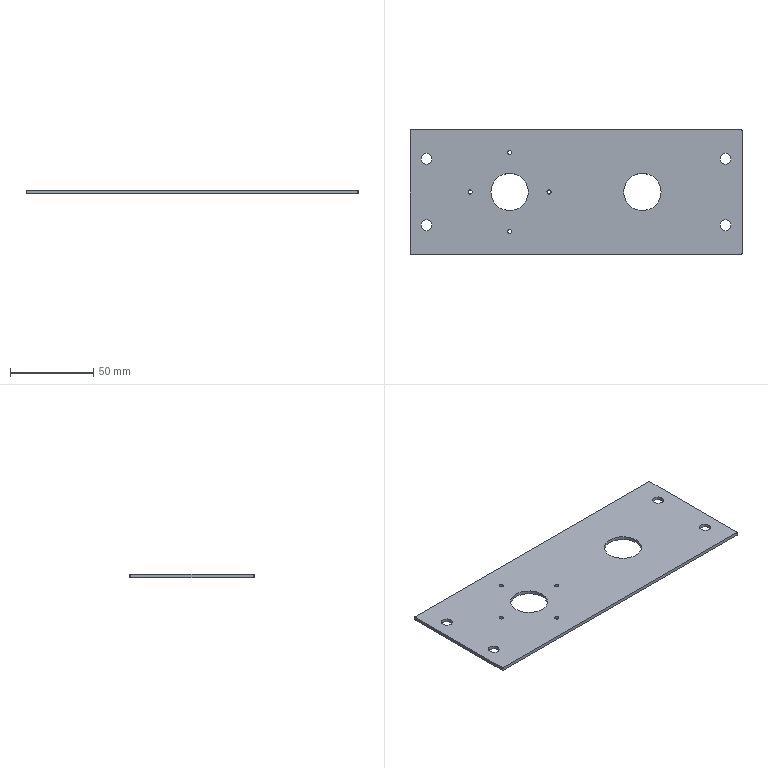Part | NX | 1 solid | 20 faces | box 200 x 75 x 2 mm | volume 28104 mm3 | cylinder 14 | plane 6 | commonest cylinder face diameters 1 x4 2.5 x4 6.5 x4 22.5 x2
STEP:
#1=CARTESIAN_POINT('',(100.,-37.,2.));
#2=VERTEX_POINT('',#1);
#3=CARTESIAN_POINT('',(100.,37.,2.));
#4=VERTEX_POINT('',#3);
#5=CARTESIAN_POINT('',(100.,-37.5,2.));
#6=DIRECTION('',(0.,1.,0.));
#7=VECTOR('',#6,1000.);
#8=LINE('',#5,#7);
#9=EDGE_CURVE('',#2,#4,#8,.T.);
#10=ORIENTED_EDGE('',*,*,#9,.F.);
#11=CARTESIAN_POINT('',(100.,-37.,0.));
#12=VERTEX_POINT('',#11);
#13=CARTESIAN_POINT('',(100.,-37.,2.));
#14=DIRECTION('',(0.,0.,-1.));
#15=VECTOR('',#14,1000.);
#16=LINE('',#13,#15);
#17=EDGE_CURVE('',#2,#12,#16,.T.);
#18=ORIENTED_EDGE('',*,*,#17,.T.);
#19=CARTESIAN_POINT('',(100.,37.,0.));
#20=VERTEX_POINT('',#19);
#21=CARTESIAN_POINT('',(100.,-37.5,0.));
#22=DIRECTION('',(0.,1.,0.));
#23=VECTOR('',#22,1000.);
#24=LINE('',#21,#23);
#25=EDGE_CURVE('',#12,#20,#24,.T.);
#26=ORIENTED_EDGE('',*,*,#25,.T.);
#27=CARTESIAN_POINT('',(100.,37.,2.));
#28=DIRECTION('',(0.,0.,-1.));
#29=VECTOR('',#28,1000.);
#30=LINE('',#27,#29);
#31=EDGE_CURVE('',#20,#4,#30,.F.);
#32=ORIENTED_EDGE('',*,*,#31,.T.);
#33=EDGE_LOOP('',(#10,#18,#26,#32));
#34=FACE_BOUND('',#33,.T.);
#35=CARTESIAN_POINT('',(100.,-37.5,2.));
#36=DIRECTION('',(-1.,0.,0.));
#37=DIRECTION('',(0.,0.,1.));
#38=AXIS2_PLACEMENT_3D('',#35,#36,#37);
#39=PLANE('',#38);
#40=ADVANCED_FACE('',(#34),#39,.F.);
#41=CARTESIAN_POINT('',(99.5,37.5,0.));
#42=VERTEX_POINT('',#41);
#43=CARTESIAN_POINT('',(-99.5,37.5,0.));
#44=VERTEX_POINT('',#43);
#45=CARTESIAN_POINT('',(-100.,37.5,0.));
#46=DIRECTION('',(-1.,0.,0.));
#47=VECTOR('',#46,1000.);
#48=LINE('',#45,#47);
#49=EDGE_CURVE('',#42,#44,#48,.T.);
#50=ORIENTED_EDGE('',*,*,#49,.T.);
#51=CARTESIAN_POINT('',(-99.5,37.5,2.));
#52=VERTEX_POINT('',#51);
#53=CARTESIAN_POINT('',(-99.5,37.5,2.));
#54=DIRECTION('',(0.,0.,-1.));
#55=VECTOR('',#54,1000.);
#56=LINE('',#53,#55);
#57=EDGE_CURVE('',#44,#52,#56,.F.);
#58=ORIENTED_EDGE('',*,*,#57,.T.);
#59=CARTESIAN_POINT('',(99.5,37.5,2.));
#60=VERTEX_POINT('',#59);
#61=CARTESIAN_POINT('',(-100.,37.5,2.));
#62=DIRECTION('',(-1.,0.,0.));
#63=VECTOR('',#62,1000.);
#64=LINE('',#61,#63);
#65=EDGE_CURVE('',#60,#52,#64,.T.);
#66=ORIENTED_EDGE('',*,*,#65,.F.);
#67=CARTESIAN_POINT('',(99.5,37.5,2.));
#68=DIRECTION('',(0.,0.,-1.));
#69=VECTOR('',#68,1000.);
#70=LINE('',#67,#69);
#71=EDGE_CURVE('',#60,#42,#70,.T.);
#72=ORIENTED_EDGE('',*,*,#71,.T.);
#73=EDGE_LOOP('',(#50,#58,#66,#72));
#74=FACE_BOUND('',#73,.T.);
#75=CARTESIAN_POINT('',(-100.,37.5,2.));
#76=DIRECTION('',(0.,-1.,0.));
#77=DIRECTION('',(0.,0.,-1.));
#78=AXIS2_PLACEMENT_3D('',#75,#76,#77);
#79=PLANE('',#78);
#80=ADVANCED_FACE('',(#74),#79,.F.);
#81=CARTESIAN_POINT('',(-100.,37.,0.));
#82=VERTEX_POINT('',#81);
#83=CARTESIAN_POINT('',(-100.,-37.,0.));
#84=VERTEX_POINT('',#83);
#85=CARTESIAN_POINT('',(-100.,-37.5,0.));
#86=DIRECTION('',(0.,-1.,0.));
#87=VECTOR('',#86,1000.);
#88=LINE('',#85,#87);
#89=EDGE_CURVE('',#82,#84,#88,.T.);
#90=ORIENTED_EDGE('',*,*,#89,.T.);
#91=CARTESIAN_POINT('',(-100.,-37.,2.));
#92=VERTEX_POINT('',#91);
#93=CARTESIAN_POINT('',(-100.,-37.,2.));
#94=DIRECTION('',(0.,0.,-1.));
#95=VECTOR('',#94,1000.);
#96=LINE('',#93,#95);
#97=EDGE_CURVE('',#84,#92,#96,.F.);
#98=ORIENTED_EDGE('',*,*,#97,.T.);
#99=CARTESIAN_POINT('',(-100.,37.,2.));
#100=VERTEX_POINT('',#99);
#101=CARTESIAN_POINT('',(-100.,-37.5,2.));
#102=DIRECTION('',(0.,-1.,0.));
#103=VECTOR('',#102,1000.);
#104=LINE('',#101,#103);
#105=EDGE_CURVE('',#100,#92,#104,.T.);
#106=ORIENTED_EDGE('',*,*,#105,.F.);
#107=CARTESIAN_POINT('',(-100.,37.,2.));
#108=DIRECTION('',(0.,0.,-1.));
#109=VECTOR('',#108,1000.);
#110=LINE('',#107,#109);
#111=EDGE_CURVE('',#100,#82,#110,.T.);
#112=ORIENTED_EDGE('',*,*,#111,.T.);
#113=EDGE_LOOP('',(#90,#98,#106,#112));
#114=FACE_BOUND('',#113,.T.);
#115=CARTESIAN_POINT('',(-100.,-37.5,2.));
#116=DIRECTION('',(1.,0.,0.));
#117=DIRECTION('',(0.,0.,-1.));
#118=AXIS2_PLACEMENT_3D('',#115,#116,#117);
#119=PLANE('',#118);
#120=ADVANCED_FACE('',(#114),#119,.F.);
#121=CARTESIAN_POINT('',(-99.5,-37.5,2.));
#122=VERTEX_POINT('',#121);
#123=CARTESIAN_POINT('',(99.5,-37.5,2.));
#124=VERTEX_POINT('',#123);
#125=CARTESIAN_POINT('',(-100.,-37.5,2.));
#126=DIRECTION('',(1.,0.,0.));
#127=VECTOR('',#126,1000.);
#128=LINE('',#125,#127);
#129=EDGE_CURVE('',#122,#124,#128,.T.);
#130=ORIENTED_EDGE('',*,*,#129,.F.);
#131=CARTESIAN_POINT('',(-99.5,-37.5,0.));
#132=VERTEX_POINT('',#131);
#133=CARTESIAN_POINT('',(-99.5,-37.5,2.));
#134=DIRECTION('',(0.,0.,-1.));
#135=VECTOR('',#134,1000.);
#136=LINE('',#133,#135);
#137=EDGE_CURVE('',#122,#132,#136,.T.);
#138=ORIENTED_EDGE('',*,*,#137,.T.);
#139=CARTESIAN_POINT('',(99.5,-37.5,0.));
#140=VERTEX_POINT('',#139);
#141=CARTESIAN_POINT('',(-100.,-37.5,0.));
#142=DIRECTION('',(1.,0.,0.));
#143=VECTOR('',#142,1000.);
#144=LINE('',#141,#143);
#145=EDGE_CURVE('',#132,#140,#144,.T.);
#146=ORIENTED_EDGE('',*,*,#145,.T.);
#147=CARTESIAN_POINT('',(99.5,-37.5,2.));
#148=DIRECTION('',(0.,0.,-1.));
#149=VECTOR('',#148,1000.);
#150=LINE('',#147,#149);
#151=EDGE_CURVE('',#140,#124,#150,.F.);
#152=ORIENTED_EDGE('',*,*,#151,.T.);
#153=EDGE_LOOP('',(#130,#138,#146,#152));
#154=FACE_BOUND('',#153,.T.);
#155=CARTESIAN_POINT('',(-100.,-37.5,2.));
#156=DIRECTION('',(0.,1.,0.));
#157=DIRECTION('',(0.,0.,1.));
#158=AXIS2_PLACEMENT_3D('',#155,#156,#157);
#159=PLANE('',#158);
#160=ADVANCED_FACE('',(#154),#159,.F.);
#161=CARTESIAN_POINT('',(-86.75,20.,2.));
#162=VERTEX_POINT('',#161);
#163=CARTESIAN_POINT('',(-90.,20.,2.));
#164=DIRECTION('',(0.,0.,1.));
#165=DIRECTION('',(1.,0.,0.));
#166=AXIS2_PLACEMENT_3D('',#163,#164,#165);
#167=CIRCLE('',#166,3.25);
#168=EDGE_CURVE('',#162,#162,#167,.T.);
#169=ORIENTED_EDGE('',*,*,#168,.F.);
#170=EDGE_LOOP('',(#169));
#171=FACE_BOUND('',#170,.T.);
#172=CARTESIAN_POINT('',(-86.75,-20.,2.));
#173=VERTEX_POINT('',#172);
#174=CARTESIAN_POINT('',(-90.,-20.,2.));
#175=DIRECTION('',(0.,0.,1.));
#176=DIRECTION('',(1.,0.,0.));
#177=AXIS2_PLACEMENT_3D('',#174,#175,#176);
#178=CIRCLE('',#177,3.25);
#179=EDGE_CURVE('',#173,#173,#178,.T.);
#180=ORIENTED_EDGE('',*,*,#179,.F.);
#181=EDGE_LOOP('',(#180));
#182=FACE_BOUND('',#181,.T.);
#183=CARTESIAN_POINT('',(93.25,20.,2.));
#184=VERTEX_POINT('',#183);
#185=CARTESIAN_POINT('',(90.,20.,2.));
#186=DIRECTION('',(0.,0.,1.));
#187=DIRECTION('',(1.,0.,0.));
#188=AXIS2_PLACEMENT_3D('',#185,#186,#187);
#189=CIRCLE('',#188,3.25);
#190=EDGE_CURVE('',#184,#184,#189,.T.);
#191=ORIENTED_EDGE('',*,*,#190,.F.);
#192=EDGE_LOOP('',(#191));
#193=FACE_BOUND('',#192,.T.);
#194=CARTESIAN_POINT('',(93.25,-20.,2.));
#195=VERTEX_POINT('',#194);
#196=CARTESIAN_POINT('',(90.,-20.,2.));
#197=DIRECTION('',(0.,0.,1.));
#198=DIRECTION('',(1.,0.,0.));
#199=AXIS2_PLACEMENT_3D('',#196,#197,#198);
#200=CIRCLE('',#199,3.25);
#201=EDGE_CURVE('',#195,#195,#200,.T.);
#202=ORIENTED_EDGE('',*,*,#201,.F.);
#203=EDGE_LOOP('',(#202));
#204=FACE_BOUND('',#203,.T.);
#205=CARTESIAN_POINT('',(-38.75,23.75,2.));
#206=VERTEX_POINT('',#205);
#207=CARTESIAN_POINT('',(-40.,23.75,2.));
#208=DIRECTION('',(0.,0.,1.));
#209=DIRECTION('',(1.,0.,0.));
#210=AXIS2_PLACEMENT_3D('',#207,#208,#209);
#211=CIRCLE('',#210,1.25);
#212=EDGE_CURVE('',#206,#206,#211,.T.);
#213=ORIENTED_EDGE('',*,*,#212,.F.);
#214=EDGE_LOOP('',(#213));
#215=FACE_BOUND('',#214,.T.);
#216=CARTESIAN_POINT('',(-38.75,-23.75,2.));
#217=VERTEX_POINT('',#216);
#218=CARTESIAN_POINT('',(-40.,-23.75,2.));
#219=DIRECTION('',(0.,0.,1.));
#220=DIRECTION('',(1.,0.,0.));
#221=AXIS2_PLACEMENT_3D('',#218,#219,#220);
#222=CIRCLE('',#221,1.25);
#223=EDGE_CURVE('',#217,#217,#222,.T.);
#224=ORIENTED_EDGE('',*,*,#223,.F.);
#225=EDGE_LOOP('',(#224));
#226=FACE_BOUND('',#225,.T.);
#227=CARTESIAN_POINT('',(-62.5,0.,2.));
#228=VERTEX_POINT('',#227);
#229=CARTESIAN_POINT('',(-63.75,0.,2.));
#230=DIRECTION('',(0.,0.,1.));
#231=DIRECTION('',(1.,0.,0.));
#232=AXIS2_PLACEMENT_3D('',#229,#230,#231);
#233=CIRCLE('',#232,1.25);
#234=EDGE_CURVE('',#228,#228,#233,.T.);
#235=ORIENTED_EDGE('',*,*,#234,.F.);
#236=EDGE_LOOP('',(#235));
#237=FACE_BOUND('',#236,.T.);
#238=CARTESIAN_POINT('',(-15.,0.,2.));
#239=VERTEX_POINT('',#238);
#240=CARTESIAN_POINT('',(-16.25,0.,2.));
#241=DIRECTION('',(0.,0.,1.));
#242=DIRECTION('',(1.,0.,0.));
#243=AXIS2_PLACEMENT_3D('',#240,#241,#242);
#244=CIRCLE('',#243,1.25);
#245=EDGE_CURVE('',#239,#239,#244,.T.);
#246=ORIENTED_EDGE('',*,*,#245,.F.);
#247=EDGE_LOOP('',(#246));
#248=FACE_BOUND('',#247,.T.);
#249=CARTESIAN_POINT('',(-28.75,0.,2.));
#250=VERTEX_POINT('',#249);
#251=CARTESIAN_POINT('',(-40.,0.,2.));
#252=DIRECTION('',(0.,0.,1.));
#253=DIRECTION('',(1.,0.,0.));
#254=AXIS2_PLACEMENT_3D('',#251,#252,#253);
#255=CIRCLE('',#254,11.25);
#256=EDGE_CURVE('',#250,#250,#255,.T.);
#257=ORIENTED_EDGE('',*,*,#256,.F.);
#258=EDGE_LOOP('',(#257));
#259=FACE_BOUND('',#258,.T.);
#260=CARTESIAN_POINT('',(51.25,0.,2.));
#261=VERTEX_POINT('',#260);
#262=CARTESIAN_POINT('',(40.,0.,2.));
#263=DIRECTION('',(0.,0.,1.));
#264=DIRECTION('',(1.,0.,0.));
#265=AXIS2_PLACEMENT_3D('',#262,#263,#264);
#266=CIRCLE('',#265,11.25);
#267=EDGE_CURVE('',#261,#261,#266,.T.);
#268=ORIENTED_EDGE('',*,*,#267,.F.);
#269=EDGE_LOOP('',(#268));
#270=FACE_BOUND('',#269,.T.);
#271=ORIENTED_EDGE('',*,*,#105,.T.);
#272=CARTESIAN_POINT('',(-99.5,-37.,2.));
#273=DIRECTION('',(0.,0.,-1.));
#274=DIRECTION('',(-1.,0.,0.));
#275=AXIS2_PLACEMENT_3D('',#272,#273,#274);
#276=CIRCLE('',#275,0.5);
#277=EDGE_CURVE('',#92,#122,#276,.F.);
#278=ORIENTED_EDGE('',*,*,#277,.T.);
#279=ORIENTED_EDGE('',*,*,#129,.T.);
#280=CARTESIAN_POINT('',(99.5,-37.,2.));
#281=DIRECTION('',(0.,0.,-1.));
#282=DIRECTION('',(-1.,0.,0.));
#283=AXIS2_PLACEMENT_3D('',#280,#281,#282);
#284=CIRCLE('',#283,0.5);
#285=EDGE_CURVE('',#124,#2,#284,.F.);
#286=ORIENTED_EDGE('',*,*,#285,.T.);
#287=ORIENTED_EDGE('',*,*,#9,.T.);
#288=CARTESIAN_POINT('',(99.5,37.,2.));
#289=DIRECTION('',(0.,0.,-1.));
#290=DIRECTION('',(-1.,0.,0.));
#291=AXIS2_PLACEMENT_3D('',#288,#289,#290);
#292=CIRCLE('',#291,0.5);
#293=EDGE_CURVE('',#4,#60,#292,.F.);
#294=ORIENTED_EDGE('',*,*,#293,.T.);
#295=ORIENTED_EDGE('',*,*,#65,.T.);
#296=CARTESIAN_POINT('',(-99.5,37.,2.));
#297=DIRECTION('',(0.,0.,-1.));
#298=DIRECTION('',(-1.,0.,0.));
#299=AXIS2_PLACEMENT_3D('',#296,#297,#298);
#300=CIRCLE('',#299,0.5);
#301=EDGE_CURVE('',#52,#100,#300,.F.);
#302=ORIENTED_EDGE('',*,*,#301,.T.);
#303=EDGE_LOOP('',(#271,#278,#279,#286,#287,#294,#295,#302));
#304=FACE_BOUND('',#303,.T.);
#305=CARTESIAN_POINT('',(100.,37.5,2.));
#306=DIRECTION('',(0.,0.,-1.));
#307=DIRECTION('',(-1.,0.,0.));
#308=AXIS2_PLACEMENT_3D('',#305,#306,#307);
#309=PLANE('',#308);
#310=ADVANCED_FACE('',(#171,#182,#193,#204,#215,#226,#237,#248,#259,#270,#304),#309,.F.);
#311=CARTESIAN_POINT('',(-86.75,20.,0.));
#312=VERTEX_POINT('',#311);
#313=CARTESIAN_POINT('',(-90.,20.,0.));
#314=DIRECTION('',(0.,0.,1.));
#315=DIRECTION('',(1.,0.,0.));
#316=AXIS2_PLACEMENT_3D('',#313,#314,#315);
#317=CIRCLE('',#316,3.25);
#318=EDGE_CURVE('',#312,#312,#317,.T.);
#319=ORIENTED_EDGE('',*,*,#318,.T.);
#320=EDGE_LOOP('',(#319));
#321=FACE_BOUND('',#320,.T.);
#322=CARTESIAN_POINT('',(-86.75,-20.,0.));
#323=VERTEX_POINT('',#322);
#324=CARTESIAN_POINT('',(-90.,-20.,0.));
#325=DIRECTION('',(0.,0.,1.));
#326=DIRECTION('',(1.,0.,0.));
#327=AXIS2_PLACEMENT_3D('',#324,#325,#326);
#328=CIRCLE('',#327,3.25);
#329=EDGE_CURVE('',#323,#323,#328,.T.);
#330=ORIENTED_EDGE('',*,*,#329,.T.);
#331=EDGE_LOOP('',(#330));
#332=FACE_BOUND('',#331,.T.);
#333=CARTESIAN_POINT('',(93.25,20.,0.));
#334=VERTEX_POINT('',#333);
#335=CARTESIAN_POINT('',(90.,20.,0.));
#336=DIRECTION('',(0.,0.,1.));
#337=DIRECTION('',(1.,0.,0.));
#338=AXIS2_PLACEMENT_3D('',#335,#336,#337);
#339=CIRCLE('',#338,3.25);
#340=EDGE_CURVE('',#334,#334,#339,.T.);
#341=ORIENTED_EDGE('',*,*,#340,.T.);
#342=EDGE_LOOP('',(#341));
#343=FACE_BOUND('',#342,.T.);
#344=CARTESIAN_POINT('',(93.25,-20.,0.));
#345=VERTEX_POINT('',#344);
#346=CARTESIAN_POINT('',(90.,-20.,0.));
#347=DIRECTION('',(0.,0.,1.));
#348=DIRECTION('',(1.,0.,0.));
#349=AXIS2_PLACEMENT_3D('',#346,#347,#348);
#350=CIRCLE('',#349,3.25);
#351=EDGE_CURVE('',#345,#345,#350,.T.);
#352=ORIENTED_EDGE('',*,*,#351,.T.);
#353=EDGE_LOOP('',(#352));
#354=FACE_BOUND('',#353,.T.);
#355=CARTESIAN_POINT('',(-41.25,23.75,0.));
#356=VERTEX_POINT('',#355);
#357=CARTESIAN_POINT('',(-40.,23.75,0.));
#358=DIRECTION('',(0.,0.,-1.));
#359=DIRECTION('',(-1.,0.,0.));
#360=AXIS2_PLACEMENT_3D('',#357,#358,#359);
#361=CIRCLE('',#360,1.25);
#362=EDGE_CURVE('',#356,#356,#361,.T.);
#363=ORIENTED_EDGE('',*,*,#362,.F.);
#364=EDGE_LOOP('',(#363));
#365=FACE_BOUND('',#364,.T.);
#366=CARTESIAN_POINT('',(-41.25,-23.75,0.));
#367=VERTEX_POINT('',#366);
#368=CARTESIAN_POINT('',(-40.,-23.75,0.));
#369=DIRECTION('',(0.,0.,-1.));
#370=DIRECTION('',(-1.,0.,0.));
#371=AXIS2_PLACEMENT_3D('',#368,#369,#370);
#372=CIRCLE('',#371,1.25);
#373=EDGE_CURVE('',#367,#367,#372,.T.);
#374=ORIENTED_EDGE('',*,*,#373,.F.);
#375=EDGE_LOOP('',(#374));
#376=FACE_BOUND('',#375,.T.);
#377=CARTESIAN_POINT('',(-65.,0.,0.));
#378=VERTEX_POINT('',#377);
#379=CARTESIAN_POINT('',(-63.75,0.,0.));
#380=DIRECTION('',(0.,0.,-1.));
#381=DIRECTION('',(-1.,0.,0.));
#382=AXIS2_PLACEMENT_3D('',#379,#380,#381);
#383=CIRCLE('',#382,1.25);
#384=EDGE_CURVE('',#378,#378,#383,.T.);
#385=ORIENTED_EDGE('',*,*,#384,.F.);
#386=EDGE_LOOP('',(#385));
#387=FACE_BOUND('',#386,.T.);
#388=CARTESIAN_POINT('',(-17.5,0.,0.));
#389=VERTEX_POINT('',#388);
#390=CARTESIAN_POINT('',(-16.25,0.,0.));
#391=DIRECTION('',(0.,0.,-1.));
#392=DIRECTION('',(-1.,0.,0.));
#393=AXIS2_PLACEMENT_3D('',#390,#391,#392);
#394=CIRCLE('',#393,1.25);
#395=EDGE_CURVE('',#389,#389,#394,.T.);
#396=ORIENTED_EDGE('',*,*,#395,.F.);
#397=EDGE_LOOP('',(#396));
#398=FACE_BOUND('',#397,.T.);
#399=CARTESIAN_POINT('',(-51.25,0.,0.));
#400=VERTEX_POINT('',#399);
#401=CARTESIAN_POINT('',(-40.,0.,0.));
#402=DIRECTION('',(0.,0.,-1.));
#403=DIRECTION('',(-1.,0.,0.));
#404=AXIS2_PLACEMENT_3D('',#401,#402,#403);
#405=CIRCLE('',#404,11.25);
#406=EDGE_CURVE('',#400,#400,#405,.T.);
#407=ORIENTED_EDGE('',*,*,#406,.F.);
#408=EDGE_LOOP('',(#407));
#409=FACE_BOUND('',#408,.T.);
#410=CARTESIAN_POINT('',(28.75,0.,0.));
#411=VERTEX_POINT('',#410);
#412=CARTESIAN_POINT('',(40.,0.,0.));
#413=DIRECTION('',(0.,0.,-1.));
#414=DIRECTION('',(-1.,0.,0.));
#415=AXIS2_PLACEMENT_3D('',#412,#413,#414);
#416=CIRCLE('',#415,11.25);
#417=EDGE_CURVE('',#411,#411,#416,.T.);
#418=ORIENTED_EDGE('',*,*,#417,.F.);
#419=EDGE_LOOP('',(#418));
#420=FACE_BOUND('',#419,.T.);
#421=ORIENTED_EDGE('',*,*,#145,.F.);
#422=CARTESIAN_POINT('',(-99.5,-37.,0.));
#423=DIRECTION('',(0.,0.,-1.));
#424=DIRECTION('',(-1.,0.,0.));
#425=AXIS2_PLACEMENT_3D('',#422,#423,#424);
#426=CIRCLE('',#425,0.5);
#427=EDGE_CURVE('',#132,#84,#426,.T.);
#428=ORIENTED_EDGE('',*,*,#427,.T.);
#429=ORIENTED_EDGE('',*,*,#89,.F.);
#430=CARTESIAN_POINT('',(-99.5,37.,0.));
#431=DIRECTION('',(0.,0.,-1.));
#432=DIRECTION('',(-1.,0.,0.));
#433=AXIS2_PLACEMENT_3D('',#430,#431,#432);
#434=CIRCLE('',#433,0.5);
#435=EDGE_CURVE('',#82,#44,#434,.T.);
#436=ORIENTED_EDGE('',*,*,#435,.T.);
#437=ORIENTED_EDGE('',*,*,#49,.F.);
#438=CARTESIAN_POINT('',(99.5,37.,0.));
#439=DIRECTION('',(0.,0.,-1.));
#440=DIRECTION('',(-1.,0.,0.));
#441=AXIS2_PLACEMENT_3D('',#438,#439,#440);
#442=CIRCLE('',#441,0.5);
#443=EDGE_CURVE('',#42,#20,#442,.T.);
#444=ORIENTED_EDGE('',*,*,#443,.T.);
#445=ORIENTED_EDGE('',*,*,#25,.F.);
#446=CARTESIAN_POINT('',(99.5,-37.,0.));
#447=DIRECTION('',(0.,0.,-1.));
#448=DIRECTION('',(-1.,0.,0.));
#449=AXIS2_PLACEMENT_3D('',#446,#447,#448);
#450=CIRCLE('',#449,0.5);
#451=EDGE_CURVE('',#12,#140,#450,.T.);
#452=ORIENTED_EDGE('',*,*,#451,.T.);
#453=EDGE_LOOP('',(#421,#428,#429,#436,#437,#444,#445,#452));
#454=FACE_BOUND('',#453,.T.);
#455=CARTESIAN_POINT('',(100.,37.5,0.));
#456=DIRECTION('',(0.,0.,-1.));
#457=DIRECTION('',(-1.,0.,0.));
#458=AXIS2_PLACEMENT_3D('',#455,#456,#457);
#459=PLANE('',#458);
#460=ADVANCED_FACE('',(#321,#332,#343,#354,#365,#376,#387,#398,#409,#420,#454),#459,.T.);
#461=ORIENTED_EDGE('',*,*,#277,.F.);
#462=ORIENTED_EDGE('',*,*,#97,.F.);
#463=ORIENTED_EDGE('',*,*,#427,.F.);
#464=ORIENTED_EDGE('',*,*,#137,.F.);
#465=EDGE_LOOP('',(#461,#462,#463,#464));
#466=FACE_BOUND('',#465,.T.);
#467=CARTESIAN_POINT('',(-99.5,-37.,2.));
#468=DIRECTION('',(0.,0.,-1.));
#469=DIRECTION('',(-1.,0.,0.));
#470=AXIS2_PLACEMENT_3D('',#467,#468,#469);
#471=CYLINDRICAL_SURFACE('',#470,0.5);
#472=ADVANCED_FACE('',(#466),#471,.T.);
#473=ORIENTED_EDGE('',*,*,#301,.F.);
#474=ORIENTED_EDGE('',*,*,#57,.F.);
#475=ORIENTED_EDGE('',*,*,#435,.F.);
#476=ORIENTED_EDGE('',*,*,#111,.F.);
#477=EDGE_LOOP('',(#473,#474,#475,#476));
#478=FACE_BOUND('',#477,.T.);
#479=CARTESIAN_POINT('',(-99.5,37.,2.));
#480=DIRECTION('',(0.,0.,-1.));
#481=DIRECTION('',(-1.,0.,0.));
#482=AXIS2_PLACEMENT_3D('',#479,#480,#481);
#483=CYLINDRICAL_SURFACE('',#482,0.5);
#484=ADVANCED_FACE('',(#478),#483,.T.);
#485=ORIENTED_EDGE('',*,*,#285,.F.);
#486=ORIENTED_EDGE('',*,*,#151,.F.);
#487=ORIENTED_EDGE('',*,*,#451,.F.);
#488=ORIENTED_EDGE('',*,*,#17,.F.);
#489=EDGE_LOOP('',(#485,#486,#487,#488));
#490=FACE_BOUND('',#489,.T.);
#491=CARTESIAN_POINT('',(99.5,-37.,2.));
#492=DIRECTION('',(0.,0.,-1.));
#493=DIRECTION('',(-1.,0.,0.));
#494=AXIS2_PLACEMENT_3D('',#491,#492,#493);
#495=CYLINDRICAL_SURFACE('',#494,0.5);
#496=ADVANCED_FACE('',(#490),#495,.T.);
#497=ORIENTED_EDGE('',*,*,#293,.F.);
#498=ORIENTED_EDGE('',*,*,#31,.F.);
#499=ORIENTED_EDGE('',*,*,#443,.F.);
#500=ORIENTED_EDGE('',*,*,#71,.F.);
#501=EDGE_LOOP('',(#497,#498,#499,#500));
#502=FACE_BOUND('',#501,.T.);
#503=CARTESIAN_POINT('',(99.5,37.,2.));
#504=DIRECTION('',(0.,0.,-1.));
#505=DIRECTION('',(-1.,0.,0.));
#506=AXIS2_PLACEMENT_3D('',#503,#504,#505);
#507=CYLINDRICAL_SURFACE('',#506,0.5);
#508=ADVANCED_FACE('',(#502),#507,.T.);
#509=ORIENTED_EDGE('',*,*,#417,.T.);
#510=EDGE_LOOP('',(#509));
#511=FACE_BOUND('',#510,.T.);
#512=ORIENTED_EDGE('',*,*,#267,.T.);
#513=EDGE_LOOP('',(#512));
#514=FACE_BOUND('',#513,.T.);
#515=CARTESIAN_POINT('',(40.,0.,-8.));
#516=DIRECTION('',(0.,0.,1.));
#517=DIRECTION('',(1.,0.,0.));
#518=AXIS2_PLACEMENT_3D('',#515,#516,#517);
#519=CYLINDRICAL_SURFACE('',#518,11.25);
#520=ADVANCED_FACE('',(#511,#514),#519,.F.);
#521=ORIENTED_EDGE('',*,*,#406,.T.);
#522=EDGE_LOOP('',(#521));
#523=FACE_BOUND('',#522,.T.);
#524=ORIENTED_EDGE('',*,*,#256,.T.);
#525=EDGE_LOOP('',(#524));
#526=FACE_BOUND('',#525,.T.);
#527=CARTESIAN_POINT('',(-40.,0.,-8.));
#528=DIRECTION('',(0.,0.,1.));
#529=DIRECTION('',(1.,0.,0.));
#530=AXIS2_PLACEMENT_3D('',#527,#528,#529);
#531=CYLINDRICAL_SURFACE('',#530,11.25);
#532=ADVANCED_FACE('',(#523,#526),#531,.F.);
#533=ORIENTED_EDGE('',*,*,#395,.T.);
#534=EDGE_LOOP('',(#533));
#535=FACE_BOUND('',#534,.T.);
#536=ORIENTED_EDGE('',*,*,#245,.T.);
#537=EDGE_LOOP('',(#536));
#538=FACE_BOUND('',#537,.T.);
#539=CARTESIAN_POINT('',(-16.25,0.,2.));
#540=DIRECTION('',(0.,0.,1.));
#541=DIRECTION('',(1.,0.,0.));
#542=AXIS2_PLACEMENT_3D('',#539,#540,#541);
#543=CYLINDRICAL_SURFACE('',#542,1.25);
#544=ADVANCED_FACE('',(#535,#538),#543,.F.);
#545=ORIENTED_EDGE('',*,*,#384,.T.);
#546=EDGE_LOOP('',(#545));
#547=FACE_BOUND('',#546,.T.);
#548=ORIENTED_EDGE('',*,*,#234,.T.);
#549=EDGE_LOOP('',(#548));
#550=FACE_BOUND('',#549,.T.);
#551=CARTESIAN_POINT('',(-63.75,0.,2.));
#552=DIRECTION('',(0.,0.,1.));
#553=DIRECTION('',(1.,0.,0.));
#554=AXIS2_PLACEMENT_3D('',#551,#552,#553);
#555=CYLINDRICAL_SURFACE('',#554,1.25);
#556=ADVANCED_FACE('',(#547,#550),#555,.F.);
#557=ORIENTED_EDGE('',*,*,#373,.T.);
#558=EDGE_LOOP('',(#557));
#559=FACE_BOUND('',#558,.T.);
#560=ORIENTED_EDGE('',*,*,#223,.T.);
#561=EDGE_LOOP('',(#560));
#562=FACE_BOUND('',#561,.T.);
#563=CARTESIAN_POINT('',(-40.,-23.75,2.));
#564=DIRECTION('',(0.,0.,1.));
#565=DIRECTION('',(1.,0.,0.));
#566=AXIS2_PLACEMENT_3D('',#563,#564,#565);
#567=CYLINDRICAL_SURFACE('',#566,1.25);
#568=ADVANCED_FACE('',(#559,#562),#567,.F.);
#569=ORIENTED_EDGE('',*,*,#362,.T.);
#570=EDGE_LOOP('',(#569));
#571=FACE_BOUND('',#570,.T.);
#572=ORIENTED_EDGE('',*,*,#212,.T.);
#573=EDGE_LOOP('',(#572));
#574=FACE_BOUND('',#573,.T.);
#575=CARTESIAN_POINT('',(-40.,23.75,2.));
#576=DIRECTION('',(0.,0.,1.));
#577=DIRECTION('',(1.,0.,0.));
#578=AXIS2_PLACEMENT_3D('',#575,#576,#577);
#579=CYLINDRICAL_SURFACE('',#578,1.25);
#580=ADVANCED_FACE('',(#571,#574),#579,.F.);
#581=ORIENTED_EDGE('',*,*,#351,.F.);
#582=EDGE_LOOP('',(#581));
#583=FACE_BOUND('',#582,.T.);
#584=ORIENTED_EDGE('',*,*,#201,.T.);
#585=EDGE_LOOP('',(#584));
#586=FACE_BOUND('',#585,.T.);
#587=CARTESIAN_POINT('',(90.,-20.,2.));
#588=DIRECTION('',(0.,0.,1.));
#589=DIRECTION('',(1.,0.,0.));
#590=AXIS2_PLACEMENT_3D('',#587,#588,#589);
#591=CYLINDRICAL_SURFACE('',#590,3.25);
#592=ADVANCED_FACE('',(#583,#586),#591,.F.);
#593=ORIENTED_EDGE('',*,*,#340,.F.);
#594=EDGE_LOOP('',(#593));
#595=FACE_BOUND('',#594,.T.);
#596=ORIENTED_EDGE('',*,*,#190,.T.);
#597=EDGE_LOOP('',(#596));
#598=FACE_BOUND('',#597,.T.);
#599=CARTESIAN_POINT('',(90.,20.,2.));
#600=DIRECTION('',(0.,0.,1.));
#601=DIRECTION('',(1.,0.,0.));
#602=AXIS2_PLACEMENT_3D('',#599,#600,#601);
#603=CYLINDRICAL_SURFACE('',#602,3.25);
#604=ADVANCED_FACE('',(#595,#598),#603,.F.);
#605=ORIENTED_EDGE('',*,*,#329,.F.);
#606=EDGE_LOOP('',(#605));
#607=FACE_BOUND('',#606,.T.);
#608=ORIENTED_EDGE('',*,*,#179,.T.);
#609=EDGE_LOOP('',(#608));
#610=FACE_BOUND('',#609,.T.);
#611=CARTESIAN_POINT('',(-90.,-20.,2.));
#612=DIRECTION('',(0.,0.,1.));
#613=DIRECTION('',(1.,0.,0.));
#614=AXIS2_PLACEMENT_3D('',#611,#612,#613);
#615=CYLINDRICAL_SURFACE('',#614,3.25);
#616=ADVANCED_FACE('',(#607,#610),#615,.F.);
#617=ORIENTED_EDGE('',*,*,#318,.F.);
#618=EDGE_LOOP('',(#617));
#619=FACE_BOUND('',#618,.T.);
#620=ORIENTED_EDGE('',*,*,#168,.T.);
#621=EDGE_LOOP('',(#620));
#622=FACE_BOUND('',#621,.T.);
#623=CARTESIAN_POINT('',(-90.,20.,2.));
#624=DIRECTION('',(0.,0.,1.));
#625=DIRECTION('',(1.,0.,0.));
#626=AXIS2_PLACEMENT_3D('',#623,#624,#625);
#627=CYLINDRICAL_SURFACE('',#626,3.25);
#628=ADVANCED_FACE('',(#619,#622),#627,.F.);
#629=CLOSED_SHELL('',(#40,#80,#120,#160,#310,#460,#472,#484,#496,#508,#520,#532,#544,#556,#568,#580,#592,#604,#616,#628));
#630=MANIFOLD_SOLID_BREP('',#629);
#631=(LENGTH_UNIT()NAMED_UNIT(*)SI_UNIT(.MILLI.,.METRE.));
#632=UNCERTAINTY_MEASURE_WITH_UNIT(LENGTH_MEASURE(0.00001),#631,'','');
#633=(NAMED_UNIT(*)PLANE_ANGLE_UNIT()SI_UNIT($,.RADIAN.));
#634=(NAMED_UNIT(*)SI_UNIT($,.STERADIAN.)SOLID_ANGLE_UNIT());
#635=(GEOMETRIC_REPRESENTATION_CONTEXT(3)GLOBAL_UNCERTAINTY_ASSIGNED_CONTEXT((#632))GLOBAL_UNIT_ASSIGNED_CONTEXT((#631,#633,#634))REPRESENTATION_CONTEXT('',''));
#636=ADVANCED_BREP_SHAPE_REPRESENTATION('',(#630),#635);